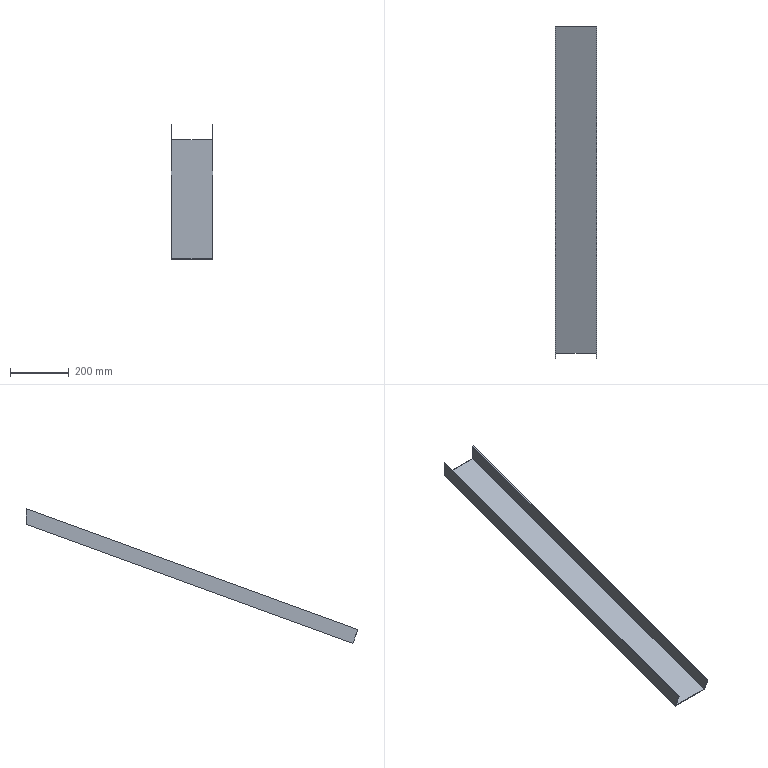Part | NX | features solid 2 | 1 solid | 10 faces | box 140 x 1127 x 457.216 mm | volume 559463 mm3 | plane 10
STEP:
#1=CARTESIAN_POINT('',(-930.,85.,-186.054));
#2=VERTEX_POINT('',#1);
#3=CARTESIAN_POINT('',(-928.,85.,-186.054));
#4=VERTEX_POINT('',#3);
#5=CARTESIAN_POINT('',(-895.,85.,-186.054));
#6=DIRECTION('',(1.,0.,0.));
#7=VECTOR('',#6,1000.);
#8=LINE('',#5,#7);
#9=EDGE_CURVE('',#2,#4,#8,.T.);
#10=ORIENTED_EDGE('',*,*,#9,.T.);
#11=CARTESIAN_POINT('',(-928.,85.,-237.135));
#12=VERTEX_POINT('',#11);
#13=CARTESIAN_POINT('',(-928.,85.,-415.937));
#14=DIRECTION('',(0.,0.,-1.));
#15=VECTOR('',#14,1000.);
#16=LINE('',#13,#15);
#17=EDGE_CURVE('',#4,#12,#16,.T.);
#18=ORIENTED_EDGE('',*,*,#17,.T.);
#19=CARTESIAN_POINT('',(-792.,85.,-237.135));
#20=VERTEX_POINT('',#19);
#21=CARTESIAN_POINT('',(-895.,85.,-237.135));
#22=DIRECTION('',(1.,0.,0.));
#23=VECTOR('',#22,1000.);
#24=LINE('',#21,#23);
#25=EDGE_CURVE('',#12,#20,#24,.T.);
#26=ORIENTED_EDGE('',*,*,#25,.T.);
#27=CARTESIAN_POINT('',(-792.,85.,-186.054));
#28=VERTEX_POINT('',#27);
#29=CARTESIAN_POINT('',(-792.,85.,-160.));
#30=DIRECTION('',(0.,0.,-1.));
#31=VECTOR('',#30,1000.);
#32=LINE('',#29,#31);
#33=EDGE_CURVE('',#28,#20,#32,.T.);
#34=ORIENTED_EDGE('',*,*,#33,.F.);
#35=CARTESIAN_POINT('',(-790.,85.,-186.054));
#36=VERTEX_POINT('',#35);
#37=CARTESIAN_POINT('',(-895.,85.,-186.054));
#38=DIRECTION('',(1.,0.,0.));
#39=VECTOR('',#38,1000.);
#40=LINE('',#37,#39);
#41=EDGE_CURVE('',#28,#36,#40,.T.);
#42=ORIENTED_EDGE('',*,*,#41,.T.);
#43=CARTESIAN_POINT('',(-790.,85.,-239.263));
#44=VERTEX_POINT('',#43);
#45=CARTESIAN_POINT('',(-790.,85.,-160.));
#46=DIRECTION('',(0.,0.,-1.));
#47=VECTOR('',#46,1000.);
#48=LINE('',#45,#47);
#49=EDGE_CURVE('',#36,#44,#48,.T.);
#50=ORIENTED_EDGE('',*,*,#49,.T.);
#51=CARTESIAN_POINT('',(-930.,85.,-239.263));
#52=VERTEX_POINT('',#51);
#53=CARTESIAN_POINT('',(-895.,85.,-239.263));
#54=DIRECTION('',(1.,0.,0.));
#55=VECTOR('',#54,1000.);
#56=LINE('',#53,#55);
#57=EDGE_CURVE('',#52,#44,#56,.T.);
#58=ORIENTED_EDGE('',*,*,#57,.F.);
#59=CARTESIAN_POINT('',(-930.,85.,-415.937));
#60=DIRECTION('',(0.,0.,-1.));
#61=VECTOR('',#60,1000.);
#62=LINE('',#59,#61);
#63=EDGE_CURVE('',#2,#52,#62,.T.);
#64=ORIENTED_EDGE('',*,*,#63,.F.);
#65=EDGE_LOOP('',(#10,#18,#26,#34,#42,#50,#58,#64));
#66=FACE_BOUND('',#65,.T.);
#67=CARTESIAN_POINT('',(-1820.,85.,-160.));
#68=DIRECTION('',(0.,1.,0.));
#69=DIRECTION('',(-1.,0.,0.));
#70=AXIS2_PLACEMENT_3D('',#67,#68,#69);
#71=PLANE('',#70);
#72=ADVANCED_FACE('',(#66),#71,.T.);
#73=CARTESIAN_POINT('',(-790.,-1042.101,-596.286));
#74=VERTEX_POINT('',#73);
#75=CARTESIAN_POINT('',(-792.,-1042.101,-596.286));
#76=VERTEX_POINT('',#75);
#77=CARTESIAN_POINT('',(-895.,-1042.101,-596.286));
#78=DIRECTION('',(-1.,0.,0.));
#79=VECTOR('',#78,1000.);
#80=LINE('',#77,#79);
#81=EDGE_CURVE('',#74,#76,#80,.T.);
#82=ORIENTED_EDGE('',*,*,#81,.T.);
#83=CARTESIAN_POINT('',(-792.,-1025.684,-641.391));
#84=VERTEX_POINT('',#83);
#85=CARTESIAN_POINT('',(-792.,-1042.101,-596.286));
#86=DIRECTION('',(0.,0.342,-0.9397));
#87=VECTOR('',#86,1000.);
#88=LINE('',#85,#87);
#89=EDGE_CURVE('',#76,#84,#88,.T.);
#90=ORIENTED_EDGE('',*,*,#89,.T.);
#91=CARTESIAN_POINT('',(-928.,-1025.684,-641.391));
#92=VERTEX_POINT('',#91);
#93=CARTESIAN_POINT('',(-895.,-1025.684,-641.391));
#94=DIRECTION('',(-1.,0.,0.));
#95=VECTOR('',#94,1000.);
#96=LINE('',#93,#95);
#97=EDGE_CURVE('',#84,#92,#96,.T.);
#98=ORIENTED_EDGE('',*,*,#97,.T.);
#99=CARTESIAN_POINT('',(-928.,-1042.101,-596.286));
#100=VERTEX_POINT('',#99);
#101=CARTESIAN_POINT('',(-928.,-1042.101,-596.286));
#102=DIRECTION('',(0.,0.342,-0.9397));
#103=VECTOR('',#102,1000.);
#104=LINE('',#101,#103);
#105=EDGE_CURVE('',#100,#92,#104,.T.);
#106=ORIENTED_EDGE('',*,*,#105,.F.);
#107=CARTESIAN_POINT('',(-930.,-1042.101,-596.286));
#108=VERTEX_POINT('',#107);
#109=CARTESIAN_POINT('',(-895.,-1042.101,-596.286));
#110=DIRECTION('',(-1.,0.,0.));
#111=VECTOR('',#110,1000.);
#112=LINE('',#109,#111);
#113=EDGE_CURVE('',#100,#108,#112,.T.);
#114=ORIENTED_EDGE('',*,*,#113,.T.);
#115=CARTESIAN_POINT('',(-930.,-1025.,-643.27));
#116=VERTEX_POINT('',#115);
#117=CARTESIAN_POINT('',(-930.,-1042.101,-596.286));
#118=DIRECTION('',(0.,0.342,-0.9397));
#119=VECTOR('',#118,1000.);
#120=LINE('',#117,#119);
#121=EDGE_CURVE('',#108,#116,#120,.T.);
#122=ORIENTED_EDGE('',*,*,#121,.T.);
#123=CARTESIAN_POINT('',(-790.,-1025.,-643.27));
#124=VERTEX_POINT('',#123);
#125=CARTESIAN_POINT('',(-895.,-1025.,-643.27));
#126=DIRECTION('',(-1.,0.,0.));
#127=VECTOR('',#126,1000.);
#128=LINE('',#125,#127);
#129=EDGE_CURVE('',#124,#116,#128,.T.);
#130=ORIENTED_EDGE('',*,*,#129,.F.);
#131=CARTESIAN_POINT('',(-790.,-1042.101,-596.286));
#132=DIRECTION('',(0.,0.342,-0.9397));
#133=VECTOR('',#132,1000.);
#134=LINE('',#131,#133);
#135=EDGE_CURVE('',#74,#124,#134,.T.);
#136=ORIENTED_EDGE('',*,*,#135,.F.);
#137=EDGE_LOOP('',(#82,#90,#98,#106,#114,#122,#130,#136));
#138=FACE_BOUND('',#137,.T.);
#139=CARTESIAN_POINT('',(-895.,-1042.101,-596.286));
#140=DIRECTION('',(0.,-0.9397,-0.342));
#141=DIRECTION('',(0.,0.342,-0.9397));
#142=AXIS2_PLACEMENT_3D('',#139,#140,#141);
#143=PLANE('',#142);
#144=ADVANCED_FACE('',(#138),#143,.T.);
#145=ORIENTED_EDGE('',*,*,#113,.F.);
#146=CARTESIAN_POINT('',(-928.,-546.597,-415.937));
#147=DIRECTION('',(0.,0.9397,0.342));
#148=VECTOR('',#147,1000.);
#149=LINE('',#146,#148);
#150=EDGE_CURVE('',#100,#4,#149,.T.);
#151=ORIENTED_EDGE('',*,*,#150,.T.);
#152=ORIENTED_EDGE('',*,*,#9,.F.);
#153=CARTESIAN_POINT('',(-930.,-546.597,-415.937));
#154=DIRECTION('',(0.,0.9397,0.342));
#155=VECTOR('',#154,1000.);
#156=LINE('',#153,#155);
#157=EDGE_CURVE('',#108,#2,#156,.T.);
#158=ORIENTED_EDGE('',*,*,#157,.F.);
#159=EDGE_LOOP('',(#145,#151,#152,#158));
#160=FACE_BOUND('',#159,.T.);
#161=CARTESIAN_POINT('',(-895.,-546.597,-415.937));
#162=DIRECTION('',(0.,0.342,-0.9397));
#163=DIRECTION('',(-1.,0.,0.));
#164=AXIS2_PLACEMENT_3D('',#161,#162,#163);
#165=PLANE('',#164);
#166=ADVANCED_FACE('',(#160),#165,.F.);
#167=CARTESIAN_POINT('',(-930.,-529.496,-462.921));
#168=DIRECTION('',(0.,0.9397,0.342));
#169=VECTOR('',#168,1000.);
#170=LINE('',#167,#169);
#171=EDGE_CURVE('',#116,#52,#170,.T.);
#172=ORIENTED_EDGE('',*,*,#171,.F.);
#173=ORIENTED_EDGE('',*,*,#121,.F.);
#174=ORIENTED_EDGE('',*,*,#157,.T.);
#175=ORIENTED_EDGE('',*,*,#63,.T.);
#176=EDGE_LOOP('',(#172,#173,#174,#175));
#177=FACE_BOUND('',#176,.T.);
#178=CARTESIAN_POINT('',(-930.,-546.597,-415.937));
#179=DIRECTION('',(-1.,0.,0.));
#180=DIRECTION('',(0.,0.08716,0.9962));
#181=AXIS2_PLACEMENT_3D('',#178,#179,#180);
#182=PLANE('',#181);
#183=ADVANCED_FACE('',(#177),#182,.T.);
#184=CARTESIAN_POINT('',(-790.,-529.496,-462.921));
#185=DIRECTION('',(0.,-0.9397,-0.342));
#186=VECTOR('',#185,1000.);
#187=LINE('',#184,#186);
#188=EDGE_CURVE('',#44,#124,#187,.T.);
#189=ORIENTED_EDGE('',*,*,#188,.F.);
#190=ORIENTED_EDGE('',*,*,#49,.F.);
#191=CARTESIAN_POINT('',(-790.,-546.597,-415.937));
#192=DIRECTION('',(0.,-0.9397,-0.342));
#193=VECTOR('',#192,1000.);
#194=LINE('',#191,#193);
#195=EDGE_CURVE('',#36,#74,#194,.T.);
#196=ORIENTED_EDGE('',*,*,#195,.T.);
#197=ORIENTED_EDGE('',*,*,#135,.T.);
#198=EDGE_LOOP('',(#189,#190,#196,#197));
#199=FACE_BOUND('',#198,.T.);
#200=CARTESIAN_POINT('',(-790.,-546.597,-415.937));
#201=DIRECTION('',(1.,0.,0.));
#202=DIRECTION('',(0.,-0.08716,-0.9962));
#203=AXIS2_PLACEMENT_3D('',#200,#201,#202);
#204=PLANE('',#203);
#205=ADVANCED_FACE('',(#199),#204,.T.);
#206=ORIENTED_EDGE('',*,*,#41,.F.);
#207=CARTESIAN_POINT('',(-792.,-546.597,-415.937));
#208=DIRECTION('',(0.,-0.9397,-0.342));
#209=VECTOR('',#208,1000.);
#210=LINE('',#207,#209);
#211=EDGE_CURVE('',#28,#76,#210,.T.);
#212=ORIENTED_EDGE('',*,*,#211,.T.);
#213=ORIENTED_EDGE('',*,*,#81,.F.);
#214=ORIENTED_EDGE('',*,*,#195,.F.);
#215=EDGE_LOOP('',(#206,#212,#213,#214));
#216=FACE_BOUND('',#215,.T.);
#217=CARTESIAN_POINT('',(-895.,-546.597,-415.937));
#218=DIRECTION('',(0.,0.342,-0.9397));
#219=DIRECTION('',(-1.,0.,0.));
#220=AXIS2_PLACEMENT_3D('',#217,#218,#219);
#221=PLANE('',#220);
#222=ADVANCED_FACE('',(#216),#221,.F.);
#223=ORIENTED_EDGE('',*,*,#171,.T.);
#224=ORIENTED_EDGE('',*,*,#57,.T.);
#225=ORIENTED_EDGE('',*,*,#188,.T.);
#226=ORIENTED_EDGE('',*,*,#129,.T.);
#227=EDGE_LOOP('',(#223,#224,#225,#226));
#228=FACE_BOUND('',#227,.T.);
#229=CARTESIAN_POINT('',(-895.,-529.496,-462.921));
#230=DIRECTION('',(0.,0.342,-0.9397));
#231=DIRECTION('',(-1.,0.,0.));
#232=AXIS2_PLACEMENT_3D('',#229,#230,#231);
#233=PLANE('',#232);
#234=ADVANCED_FACE('',(#228),#233,.T.);
#235=CARTESIAN_POINT('',(-928.,-530.18,-461.042));
#236=DIRECTION('',(0.,0.9397,0.342));
#237=VECTOR('',#236,1000.);
#238=LINE('',#235,#237);
#239=EDGE_CURVE('',#92,#12,#238,.T.);
#240=ORIENTED_EDGE('',*,*,#239,.T.);
#241=ORIENTED_EDGE('',*,*,#17,.F.);
#242=ORIENTED_EDGE('',*,*,#150,.F.);
#243=ORIENTED_EDGE('',*,*,#105,.T.);
#244=EDGE_LOOP('',(#240,#241,#242,#243));
#245=FACE_BOUND('',#244,.T.);
#246=CARTESIAN_POINT('',(-928.,-546.597,-415.937));
#247=DIRECTION('',(-1.,0.,0.));
#248=DIRECTION('',(0.,0.08716,0.9962));
#249=AXIS2_PLACEMENT_3D('',#246,#247,#248);
#250=PLANE('',#249);
#251=ADVANCED_FACE('',(#245),#250,.F.);
#252=CARTESIAN_POINT('',(-792.,-530.18,-461.042));
#253=DIRECTION('',(0.,-0.9397,-0.342));
#254=VECTOR('',#253,1000.);
#255=LINE('',#252,#254);
#256=EDGE_CURVE('',#20,#84,#255,.T.);
#257=ORIENTED_EDGE('',*,*,#256,.T.);
#258=ORIENTED_EDGE('',*,*,#89,.F.);
#259=ORIENTED_EDGE('',*,*,#211,.F.);
#260=ORIENTED_EDGE('',*,*,#33,.T.);
#261=EDGE_LOOP('',(#257,#258,#259,#260));
#262=FACE_BOUND('',#261,.T.);
#263=CARTESIAN_POINT('',(-792.,-546.597,-415.937));
#264=DIRECTION('',(1.,0.,0.));
#265=DIRECTION('',(0.,-0.08716,-0.9962));
#266=AXIS2_PLACEMENT_3D('',#263,#264,#265);
#267=PLANE('',#266);
#268=ADVANCED_FACE('',(#262),#267,.F.);
#269=ORIENTED_EDGE('',*,*,#239,.F.);
#270=ORIENTED_EDGE('',*,*,#97,.F.);
#271=ORIENTED_EDGE('',*,*,#256,.F.);
#272=ORIENTED_EDGE('',*,*,#25,.F.);
#273=EDGE_LOOP('',(#269,#270,#271,#272));
#274=FACE_BOUND('',#273,.T.);
#275=CARTESIAN_POINT('',(-895.,-530.18,-461.042));
#276=DIRECTION('',(0.,0.342,-0.9397));
#277=DIRECTION('',(-1.,0.,0.));
#278=AXIS2_PLACEMENT_3D('',#275,#276,#277);
#279=PLANE('',#278);
#280=ADVANCED_FACE('',(#274),#279,.F.);
#281=CLOSED_SHELL('',(#72,#144,#166,#183,#205,#222,#234,#251,#268,#280));
#282=MANIFOLD_SOLID_BREP('',#281);
#283=(LENGTH_UNIT()NAMED_UNIT(*)SI_UNIT(.MILLI.,.METRE.));
#284=UNCERTAINTY_MEASURE_WITH_UNIT(LENGTH_MEASURE(0.00001),#283,'','');
#285=(NAMED_UNIT(*)PLANE_ANGLE_UNIT()SI_UNIT($,.RADIAN.));
#286=(NAMED_UNIT(*)SI_UNIT($,.STERADIAN.)SOLID_ANGLE_UNIT());
#287=(GEOMETRIC_REPRESENTATION_CONTEXT(3)GLOBAL_UNCERTAINTY_ASSIGNED_CONTEXT((#284))GLOBAL_UNIT_ASSIGNED_CONTEXT((#283,#285,#286))REPRESENTATION_CONTEXT('',''));
#288=ADVANCED_BREP_SHAPE_REPRESENTATION('',(#282),#287);